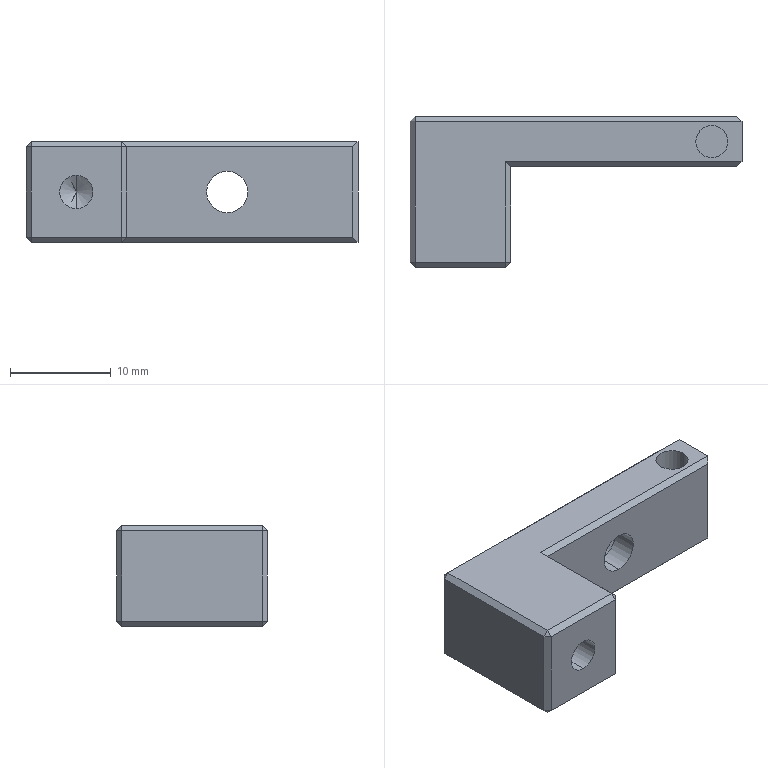Part | SolidWorks | features ICE 5, Chamfer 1, Extrusion 1, HoleWzd 1, MirrorPattern 1 | 1 solid | 44 faces | box 33 x 15 x 10 mm | volume 2355 mm3 | plane 32 | cylinder 10 | cone 2 | commonest cylinder face diameters 3.2 x4 3.3 x2 4.1 x2 7 x2
STEP:
#1=CARTESIAN_POINT('',(3.5,2.5,2.95));
#2=VERTEX_POINT('',#1);
#3=CARTESIAN_POINT('',(3.5,2.5,7.05));
#4=VERTEX_POINT('',#3);
#5=CARTESIAN_POINT('',(3.5,2.5,5.));
#6=DIRECTION('',(0.,1.,0.));
#7=DIRECTION('',(-1.,0.,0.));
#8=AXIS2_PLACEMENT_3D('',#5,#6,#7);
#9=CIRCLE('',#8,2.05);
#10=EDGE_CURVE('',#2,#4,#9,.T.);
#11=ORIENTED_EDGE('',*,*,#10,.F.);
#12=CARTESIAN_POINT('',(3.5,5.,2.95));
#13=VERTEX_POINT('',#12);
#14=CARTESIAN_POINT('',(3.5,-5.,2.95));
#15=DIRECTION('',(0.,1.,0.));
#16=VECTOR('',#15,1000.);
#17=LINE('',#14,#16);
#18=EDGE_CURVE('',#2,#13,#17,.T.);
#19=ORIENTED_EDGE('',*,*,#18,.T.);
#20=CARTESIAN_POINT('',(3.5,5.,7.05));
#21=VERTEX_POINT('',#20);
#22=CARTESIAN_POINT('',(3.5,5.,5.));
#23=DIRECTION('',(0.,1.,0.));
#24=DIRECTION('',(0.,0.,1.));
#25=AXIS2_PLACEMENT_3D('',#22,#23,#24);
#26=CIRCLE('',#25,2.05);
#27=EDGE_CURVE('',#13,#21,#26,.T.);
#28=ORIENTED_EDGE('',*,*,#27,.T.);
#29=CARTESIAN_POINT('',(3.5,-5.,7.05));
#30=DIRECTION('',(0.,1.,0.));
#31=VECTOR('',#30,1000.);
#32=LINE('',#29,#31);
#33=EDGE_CURVE('',#4,#21,#32,.T.);
#34=ORIENTED_EDGE('',*,*,#33,.F.);
#35=EDGE_LOOP('',(#11,#19,#28,#34));
#36=FACE_OUTER_BOUND('',#35,.T.);
#37=CARTESIAN_POINT('',(3.5,-5.,5.));
#38=DIRECTION('',(0.,1.,0.));
#39=DIRECTION('',(0.,0.,1.));
#40=AXIS2_PLACEMENT_3D('',#37,#38,#39);
#41=CYLINDRICAL_SURFACE('',#40,2.05);
#42=ADVANCED_FACE('',(#36),#41,.F.);
#43=CARTESIAN_POINT('',(15.1,5.,7.));
#44=VERTEX_POINT('',#43);
#45=CARTESIAN_POINT('',(11.9,5.,7.));
#46=VERTEX_POINT('',#45);
#47=CARTESIAN_POINT('',(13.5,5.,7.));
#48=DIRECTION('',(0.,0.,-1.));
#49=DIRECTION('',(-1.,0.,0.));
#50=AXIS2_PLACEMENT_3D('',#47,#48,#49);
#51=CIRCLE('',#50,1.6);
#52=EDGE_CURVE('',#44,#46,#51,.T.);
#53=ORIENTED_EDGE('',*,*,#52,.T.);
#54=CARTESIAN_POINT('',(11.9,5.,10.));
#55=VERTEX_POINT('',#54);
#56=CARTESIAN_POINT('',(11.9,5.,7.));
#57=DIRECTION('',(0.,0.,1.));
#58=VECTOR('',#57,1000.);
#59=LINE('',#56,#58);
#60=EDGE_CURVE('',#46,#55,#59,.T.);
#61=ORIENTED_EDGE('',*,*,#60,.T.);
#62=CARTESIAN_POINT('',(15.1,5.,10.));
#63=VERTEX_POINT('',#62);
#64=CARTESIAN_POINT('',(13.5,5.,10.));
#65=DIRECTION('',(0.,0.,-1.));
#66=DIRECTION('',(-1.,0.,0.));
#67=AXIS2_PLACEMENT_3D('',#64,#65,#66);
#68=CIRCLE('',#67,1.6);
#69=EDGE_CURVE('',#63,#55,#68,.T.);
#70=ORIENTED_EDGE('',*,*,#69,.F.);
#71=CARTESIAN_POINT('',(15.1,5.,7.));
#72=DIRECTION('',(0.,0.,1.));
#73=VECTOR('',#72,1000.);
#74=LINE('',#71,#73);
#75=EDGE_CURVE('',#44,#63,#74,.T.);
#76=ORIENTED_EDGE('',*,*,#75,.F.);
#77=EDGE_LOOP('',(#53,#61,#70,#76));
#78=FACE_OUTER_BOUND('',#77,.T.);
#79=CARTESIAN_POINT('',(13.5,5.,7.));
#80=DIRECTION('',(0.,0.,1.));
#81=DIRECTION('',(1.,0.,0.));
#82=AXIS2_PLACEMENT_3D('',#79,#80,#81);
#83=CYLINDRICAL_SURFACE('',#82,1.6);
#84=ADVANCED_FACE('',(#78),#83,.F.);
#85=CARTESIAN_POINT('',(15.1,5.,3.));
#86=VERTEX_POINT('',#85);
#87=CARTESIAN_POINT('',(11.9,5.,3.));
#88=VERTEX_POINT('',#87);
#89=CARTESIAN_POINT('',(13.5,5.,3.));
#90=DIRECTION('',(0.,0.,-1.));
#91=DIRECTION('',(-1.,0.,0.));
#92=AXIS2_PLACEMENT_3D('',#89,#90,#91);
#93=CIRCLE('',#92,1.6);
#94=EDGE_CURVE('',#86,#88,#93,.T.);
#95=ORIENTED_EDGE('',*,*,#94,.F.);
#96=CARTESIAN_POINT('',(15.1,5.,0.));
#97=VERTEX_POINT('',#96);
#98=CARTESIAN_POINT('',(15.1,5.,3.));
#99=DIRECTION('',(0.,0.,-1.));
#100=VECTOR('',#99,1000.);
#101=LINE('',#98,#100);
#102=EDGE_CURVE('',#86,#97,#101,.T.);
#103=ORIENTED_EDGE('',*,*,#102,.T.);
#104=CARTESIAN_POINT('',(11.9,5.,0.));
#105=VERTEX_POINT('',#104);
#106=CARTESIAN_POINT('',(13.5,5.,0.));
#107=DIRECTION('',(0.,0.,-1.));
#108=DIRECTION('',(-1.,0.,0.));
#109=AXIS2_PLACEMENT_3D('',#106,#107,#108);
#110=CIRCLE('',#109,1.6);
#111=EDGE_CURVE('',#97,#105,#110,.T.);
#112=ORIENTED_EDGE('',*,*,#111,.T.);
#113=CARTESIAN_POINT('',(11.9,5.,3.));
#114=DIRECTION('',(0.,0.,-1.));
#115=VECTOR('',#114,1000.);
#116=LINE('',#113,#115);
#117=EDGE_CURVE('',#88,#105,#116,.T.);
#118=ORIENTED_EDGE('',*,*,#117,.F.);
#119=EDGE_LOOP('',(#95,#103,#112,#118));
#120=FACE_OUTER_BOUND('',#119,.T.);
#121=CARTESIAN_POINT('',(13.5,5.,3.));
#122=DIRECTION('',(0.,0.,-1.));
#123=DIRECTION('',(-1.,0.,0.));
#124=AXIS2_PLACEMENT_3D('',#121,#122,#123);
#125=CYLINDRICAL_SURFACE('',#124,1.6);
#126=ADVANCED_FACE('',(#120),#125,.F.);
#127=CARTESIAN_POINT('',(3.5,5.,1.5));
#128=VERTEX_POINT('',#127);
#129=CARTESIAN_POINT('',(3.5,5.,8.5));
#130=VERTEX_POINT('',#129);
#131=CARTESIAN_POINT('',(3.5,5.,5.));
#132=DIRECTION('',(0.,1.,0.));
#133=DIRECTION('',(0.,0.,1.));
#134=AXIS2_PLACEMENT_3D('',#131,#132,#133);
#135=CIRCLE('',#134,3.5);
#136=EDGE_CURVE('',#128,#130,#135,.T.);
#137=ORIENTED_EDGE('',*,*,#136,.F.);
#138=CARTESIAN_POINT('',(3.5,7.5,1.5));
#139=VERTEX_POINT('',#138);
#140=CARTESIAN_POINT('',(3.5,5.,1.5));
#141=DIRECTION('',(0.,1.,0.));
#142=VECTOR('',#141,1000.);
#143=LINE('',#140,#142);
#144=EDGE_CURVE('',#128,#139,#143,.T.);
#145=ORIENTED_EDGE('',*,*,#144,.T.);
#146=CARTESIAN_POINT('',(3.5,7.5,8.5));
#147=VERTEX_POINT('',#146);
#148=CARTESIAN_POINT('',(3.5,7.5,5.));
#149=DIRECTION('',(0.,1.,0.));
#150=DIRECTION('',(0.,0.,1.));
#151=AXIS2_PLACEMENT_3D('',#148,#149,#150);
#152=CIRCLE('',#151,3.5);
#153=EDGE_CURVE('',#139,#147,#152,.T.);
#154=ORIENTED_EDGE('',*,*,#153,.T.);
#155=CARTESIAN_POINT('',(3.5,5.,8.5));
#156=DIRECTION('',(0.,1.,0.));
#157=VECTOR('',#156,1000.);
#158=LINE('',#155,#157);
#159=EDGE_CURVE('',#130,#147,#158,.T.);
#160=ORIENTED_EDGE('',*,*,#159,.F.);
#161=EDGE_LOOP('',(#137,#145,#154,#160));
#162=FACE_OUTER_BOUND('',#161,.T.);
#163=CARTESIAN_POINT('',(3.5,5.,5.));
#164=DIRECTION('',(0.,1.,0.));
#165=DIRECTION('',(0.,0.,1.));
#166=AXIS2_PLACEMENT_3D('',#163,#164,#165);
#167=CYLINDRICAL_SURFACE('',#166,3.5);
#168=ADVANCED_FACE('',(#162),#167,.F.);
#169=CARTESIAN_POINT('',(-11.5,2.6,6.65));
#170=VERTEX_POINT('',#169);
#171=CARTESIAN_POINT('',(-11.5,2.6,3.35));
#172=VERTEX_POINT('',#171);
#173=CARTESIAN_POINT('',(-11.5,2.6,5.));
#174=DIRECTION('',(0.,-1.,0.));
#175=DIRECTION('',(0.,0.,-1.));
#176=AXIS2_PLACEMENT_3D('',#173,#174,#175);
#177=CIRCLE('',#176,1.65);
#178=EDGE_CURVE('',#170,#172,#177,.T.);
#179=ORIENTED_EDGE('',*,*,#178,.F.);
#180=CARTESIAN_POINT('',(-11.5,-7.5,6.65));
#181=VERTEX_POINT('',#180);
#182=CARTESIAN_POINT('',(-11.5,-7.5,6.65));
#183=DIRECTION('',(0.,-1.,0.));
#184=VECTOR('',#183,1000.);
#185=LINE('',#182,#184);
#186=EDGE_CURVE('',#170,#181,#185,.T.);
#187=ORIENTED_EDGE('',*,*,#186,.T.);
#188=CARTESIAN_POINT('',(-11.5,-7.5,3.35));
#189=VERTEX_POINT('',#188);
#190=CARTESIAN_POINT('',(-11.5,-7.5,5.));
#191=DIRECTION('',(0.,-1.,0.));
#192=DIRECTION('',(0.,0.,-1.));
#193=AXIS2_PLACEMENT_3D('',#190,#191,#192);
#194=CIRCLE('',#193,1.65);
#195=EDGE_CURVE('',#181,#189,#194,.T.);
#196=ORIENTED_EDGE('',*,*,#195,.T.);
#197=CARTESIAN_POINT('',(-11.5,-7.5,3.35));
#198=DIRECTION('',(0.,-1.,0.));
#199=VECTOR('',#198,1000.);
#200=LINE('',#197,#199);
#201=EDGE_CURVE('',#172,#189,#200,.T.);
#202=ORIENTED_EDGE('',*,*,#201,.F.);
#203=EDGE_LOOP('',(#179,#187,#196,#202));
#204=FACE_OUTER_BOUND('',#203,.T.);
#205=CARTESIAN_POINT('',(-11.5,-7.5,5.));
#206=DIRECTION('',(0.,-1.,0.));
#207=DIRECTION('',(0.,0.,-1.));
#208=AXIS2_PLACEMENT_3D('',#205,#206,#207);
#209=CYLINDRICAL_SURFACE('',#208,1.65);
#210=ADVANCED_FACE('',(#204),#209,.F.);
#211=CARTESIAN_POINT('',(-11.5,3.591,5.));
#212=VERTEX_POINT('',#211);
#213=CARTESIAN_POINT('',(-11.5,2.6,3.35));
#214=DIRECTION('',(0.,-0.515,-0.8572));
#215=VECTOR('',#214,1000.);
#216=LINE('',#213,#215);
#217=EDGE_CURVE('',#212,#172,#216,.T.);
#218=ORIENTED_EDGE('',*,*,#217,.F.);
#219=CARTESIAN_POINT('',(-11.5,2.6,6.65));
#220=DIRECTION('',(0.,-0.515,0.8572));
#221=VECTOR('',#220,1000.);
#222=LINE('',#219,#221);
#223=EDGE_CURVE('',#212,#170,#222,.T.);
#224=ORIENTED_EDGE('',*,*,#223,.T.);
#225=ORIENTED_EDGE('',*,*,#178,.T.);
#226=EDGE_LOOP('',(#218,#224,#225));
#227=FACE_OUTER_BOUND('',#226,.T.);
#228=CARTESIAN_POINT('',(-11.5,2.6,5.));
#229=DIRECTION('',(0.,-1.,0.));
#230=DIRECTION('',(0.,0.,-1.));
#231=AXIS2_PLACEMENT_3D('',#228,#229,#230);
#232=CONICAL_SURFACE('',#231,1.65,1.03);
#233=ADVANCED_FACE('',(#227),#232,.F.);
#234=CARTESIAN_POINT('',(16.5,3.,10.));
#235=VERTEX_POINT('',#234);
#236=CARTESIAN_POINT('',(16.5,7.,10.));
#237=VERTEX_POINT('',#236);
#238=CARTESIAN_POINT('',(16.5,-7.5,10.));
#239=DIRECTION('',(0.,1.,0.));
#240=VECTOR('',#239,1000.);
#241=LINE('',#238,#240);
#242=EDGE_CURVE('',#235,#237,#241,.T.);
#243=ORIENTED_EDGE('',*,*,#242,.T.);
#244=CARTESIAN_POINT('',(-16.,7.,10.));
#245=VERTEX_POINT('',#244);
#246=CARTESIAN_POINT('',(0.,7.,10.));
#247=DIRECTION('',(-1.,0.,0.));
#248=VECTOR('',#247,1000.);
#249=LINE('',#246,#248);
#250=EDGE_CURVE('',#237,#245,#249,.T.);
#251=ORIENTED_EDGE('',*,*,#250,.T.);
#252=CARTESIAN_POINT('',(-16.,-7.,10.));
#253=VERTEX_POINT('',#252);
#254=CARTESIAN_POINT('',(-16.,0.,10.));
#255=DIRECTION('',(0.,-1.,0.));
#256=VECTOR('',#255,1000.);
#257=LINE('',#254,#256);
#258=EDGE_CURVE('',#245,#253,#257,.T.);
#259=ORIENTED_EDGE('',*,*,#258,.T.);
#260=CARTESIAN_POINT('',(-7.,-7.,10.));
#261=VERTEX_POINT('',#260);
#262=CARTESIAN_POINT('',(0.,-7.,10.));
#263=DIRECTION('',(1.,0.,0.));
#264=VECTOR('',#263,1000.);
#265=LINE('',#262,#264);
#266=EDGE_CURVE('',#253,#261,#265,.T.);
#267=ORIENTED_EDGE('',*,*,#266,.T.);
#268=CARTESIAN_POINT('',(-7.,3.,10.));
#269=VERTEX_POINT('',#268);
#270=CARTESIAN_POINT('',(-7.,0.,10.));
#271=DIRECTION('',(0.,1.,0.));
#272=VECTOR('',#271,1000.);
#273=LINE('',#270,#272);
#274=EDGE_CURVE('',#261,#269,#273,.T.);
#275=ORIENTED_EDGE('',*,*,#274,.T.);
#276=CARTESIAN_POINT('',(0.,3.,10.));
#277=DIRECTION('',(1.,0.,0.));
#278=VECTOR('',#277,1000.);
#279=LINE('',#276,#278);
#280=EDGE_CURVE('',#269,#235,#279,.T.);
#281=ORIENTED_EDGE('',*,*,#280,.T.);
#282=EDGE_LOOP('',(#243,#251,#259,#267,#275,#281));
#283=FACE_OUTER_BOUND('',#282,.T.);
#284=ORIENTED_EDGE('',*,*,#69,.T.);
#285=CARTESIAN_POINT('',(13.5,5.,10.));
#286=DIRECTION('',(0.,0.,-1.));
#287=DIRECTION('',(-1.,0.,0.));
#288=AXIS2_PLACEMENT_3D('',#285,#286,#287);
#289=CIRCLE('',#288,1.6);
#290=EDGE_CURVE('',#55,#63,#289,.T.);
#291=ORIENTED_EDGE('',*,*,#290,.T.);
#292=EDGE_LOOP('',(#284,#291));
#293=FACE_BOUND('',#292,.T.);
#294=CARTESIAN_POINT('',(0.,0.,10.));
#295=DIRECTION('',(0.,0.,-1.));
#296=DIRECTION('',(-1.,0.,0.));
#297=AXIS2_PLACEMENT_3D('',#294,#295,#296);
#298=PLANE('',#297);
#299=ADVANCED_FACE('',(#283,#293),#298,.F.);
#300=CARTESIAN_POINT('',(16.5,3.,0.));
#301=VERTEX_POINT('',#300);
#302=CARTESIAN_POINT('',(16.5,7.,0.));
#303=VERTEX_POINT('',#302);
#304=CARTESIAN_POINT('',(16.5,-7.5,0.));
#305=DIRECTION('',(0.,1.,0.));
#306=VECTOR('',#305,1000.);
#307=LINE('',#304,#306);
#308=EDGE_CURVE('',#301,#303,#307,.T.);
#309=ORIENTED_EDGE('',*,*,#308,.T.);
#310=CARTESIAN_POINT('',(16.5,7.,10.));
#311=DIRECTION('',(0.,0.,1.));
#312=VECTOR('',#311,1000.);
#313=LINE('',#310,#312);
#314=EDGE_CURVE('',#303,#237,#313,.T.);
#315=ORIENTED_EDGE('',*,*,#314,.T.);
#316=ORIENTED_EDGE('',*,*,#242,.F.);
#317=CARTESIAN_POINT('',(16.5,3.,10.));
#318=DIRECTION('',(0.,0.,-1.));
#319=VECTOR('',#318,1000.);
#320=LINE('',#317,#319);
#321=EDGE_CURVE('',#235,#301,#320,.T.);
#322=ORIENTED_EDGE('',*,*,#321,.T.);
#323=EDGE_LOOP('',(#309,#315,#316,#322));
#324=FACE_OUTER_BOUND('',#323,.T.);
#325=CARTESIAN_POINT('',(16.5,-7.5,10.));
#326=DIRECTION('',(-1.,0.,0.));
#327=DIRECTION('',(0.,0.,1.));
#328=AXIS2_PLACEMENT_3D('',#325,#326,#327);
#329=PLANE('',#328);
#330=ADVANCED_FACE('',(#324),#329,.F.);
#331=CARTESIAN_POINT('',(3.5,7.5,5.));
#332=DIRECTION('',(0.,1.,0.));
#333=DIRECTION('',(0.,0.,1.));
#334=AXIS2_PLACEMENT_3D('',#331,#332,#333);
#335=CIRCLE('',#334,3.5);
#336=EDGE_CURVE('',#147,#139,#335,.T.);
#337=ORIENTED_EDGE('',*,*,#336,.F.);
#338=ORIENTED_EDGE('',*,*,#153,.F.);
#339=EDGE_LOOP('',(#337,#338));
#340=FACE_BOUND('',#339,.T.);
#341=CARTESIAN_POINT('',(-16.,7.5,0.5));
#342=VERTEX_POINT('',#341);
#343=CARTESIAN_POINT('',(-16.,7.5,9.5));
#344=VERTEX_POINT('',#343);
#345=CARTESIAN_POINT('',(-16.,7.5,10.));
#346=DIRECTION('',(0.,0.,1.));
#347=VECTOR('',#346,1000.);
#348=LINE('',#345,#347);
#349=EDGE_CURVE('',#342,#344,#348,.T.);
#350=ORIENTED_EDGE('',*,*,#349,.T.);
#351=CARTESIAN_POINT('',(16.,7.5,9.5));
#352=VERTEX_POINT('',#351);
#353=CARTESIAN_POINT('',(-16.5,7.5,9.5));
#354=DIRECTION('',(1.,0.,0.));
#355=VECTOR('',#354,1000.);
#356=LINE('',#353,#355);
#357=EDGE_CURVE('',#344,#352,#356,.T.);
#358=ORIENTED_EDGE('',*,*,#357,.T.);
#359=CARTESIAN_POINT('',(16.,7.5,0.5));
#360=VERTEX_POINT('',#359);
#361=CARTESIAN_POINT('',(16.,7.5,10.));
#362=DIRECTION('',(0.,0.,-1.));
#363=VECTOR('',#362,1000.);
#364=LINE('',#361,#363);
#365=EDGE_CURVE('',#352,#360,#364,.T.);
#366=ORIENTED_EDGE('',*,*,#365,.T.);
#367=CARTESIAN_POINT('',(-16.5,7.5,0.5));
#368=DIRECTION('',(-1.,0.,0.));
#369=VECTOR('',#368,1000.);
#370=LINE('',#367,#369);
#371=EDGE_CURVE('',#360,#342,#370,.T.);
#372=ORIENTED_EDGE('',*,*,#371,.T.);
#373=EDGE_LOOP('',(#350,#358,#366,#372));
#374=FACE_OUTER_BOUND('',#373,.T.);
#375=CARTESIAN_POINT('',(-16.5,7.5,10.));
#376=DIRECTION('',(0.,-1.,0.));
#377=DIRECTION('',(0.,0.,-1.));
#378=AXIS2_PLACEMENT_3D('',#375,#376,#377);
#379=PLANE('',#378);
#380=ADVANCED_FACE('',(#340,#374),#379,.F.);
#381=CARTESIAN_POINT('',(-16.5,-7.,9.5));
#382=VERTEX_POINT('',#381);
#383=CARTESIAN_POINT('',(-16.5,7.,9.5));
#384=VERTEX_POINT('',#383);
#385=CARTESIAN_POINT('',(-16.5,-7.5,9.5));
#386=DIRECTION('',(0.,1.,0.));
#387=VECTOR('',#386,1000.);
#388=LINE('',#385,#387);
#389=EDGE_CURVE('',#382,#384,#388,.T.);
#390=ORIENTED_EDGE('',*,*,#389,.T.);
#391=CARTESIAN_POINT('',(-16.5,7.,0.5));
#392=VERTEX_POINT('',#391);
#393=CARTESIAN_POINT('',(-16.5,7.,10.));
#394=DIRECTION('',(0.,0.,-1.));
#395=VECTOR('',#394,1000.);
#396=LINE('',#393,#395);
#397=EDGE_CURVE('',#384,#392,#396,.T.);
#398=ORIENTED_EDGE('',*,*,#397,.T.);
#399=CARTESIAN_POINT('',(-16.5,-7.,0.5));
#400=VERTEX_POINT('',#399);
#401=CARTESIAN_POINT('',(-16.5,-7.5,0.5));
#402=DIRECTION('',(0.,-1.,0.));
#403=VECTOR('',#402,1000.);
#404=LINE('',#401,#403);
#405=EDGE_CURVE('',#392,#400,#404,.T.);
#406=ORIENTED_EDGE('',*,*,#405,.T.);
#407=CARTESIAN_POINT('',(-16.5,-7.,10.));
#408=DIRECTION('',(0.,0.,1.));
#409=VECTOR('',#408,1000.);
#410=LINE('',#407,#409);
#411=EDGE_CURVE('',#400,#382,#410,.T.);
#412=ORIENTED_EDGE('',*,*,#411,.T.);
#413=EDGE_LOOP('',(#390,#398,#406,#412));
#414=FACE_OUTER_BOUND('',#413,.T.);
#415=CARTESIAN_POINT('',(-16.5,-7.5,10.));
#416=DIRECTION('',(1.,0.,0.));
#417=DIRECTION('',(0.,0.,-1.));
#418=AXIS2_PLACEMENT_3D('',#415,#416,#417);
#419=PLANE('',#418);
#420=ADVANCED_FACE('',(#414),#419,.F.);
#421=CARTESIAN_POINT('',(-16.,-7.5,9.5));
#422=VERTEX_POINT('',#421);
#423=CARTESIAN_POINT('',(-16.,-7.5,0.5));
#424=VERTEX_POINT('',#423);
#425=CARTESIAN_POINT('',(-16.,-7.5,10.));
#426=DIRECTION('',(0.,0.,-1.));
#427=VECTOR('',#426,1000.);
#428=LINE('',#425,#427);
#429=EDGE_CURVE('',#422,#424,#428,.T.);
#430=ORIENTED_EDGE('',*,*,#429,.T.);
#431=CARTESIAN_POINT('',(-7.,-7.5,0.5));
#432=VERTEX_POINT('',#431);
#433=CARTESIAN_POINT('',(-6.5,-7.5,0.5));
#434=DIRECTION('',(1.,0.,0.));
#435=VECTOR('',#434,1000.);
#436=LINE('',#433,#435);
#437=EDGE_CURVE('',#424,#432,#436,.T.);
#438=ORIENTED_EDGE('',*,*,#437,.T.);
#439=CARTESIAN_POINT('',(-7.,-7.5,9.5));
#440=VERTEX_POINT('',#439);
#441=CARTESIAN_POINT('',(-7.,-7.5,10.));
#442=DIRECTION('',(0.,0.,1.));
#443=VECTOR('',#442,1000.);
#444=LINE('',#441,#443);
#445=EDGE_CURVE('',#432,#440,#444,.T.);
#446=ORIENTED_EDGE('',*,*,#445,.T.);
#447=CARTESIAN_POINT('',(-16.5,-7.5,9.5));
#448=DIRECTION('',(-1.,0.,0.));
#449=VECTOR('',#448,1000.);
#450=LINE('',#447,#449);
#451=EDGE_CURVE('',#440,#422,#450,.T.);
#452=ORIENTED_EDGE('',*,*,#451,.T.);
#453=EDGE_LOOP('',(#430,#438,#446,#452));
#454=FACE_OUTER_BOUND('',#453,.T.);
#455=CARTESIAN_POINT('',(-11.5,-7.5,5.));
#456=DIRECTION('',(0.,-1.,0.));
#457=DIRECTION('',(0.,0.,-1.));
#458=AXIS2_PLACEMENT_3D('',#455,#456,#457);
#459=CIRCLE('',#458,1.65);
#460=EDGE_CURVE('',#189,#181,#459,.T.);
#461=ORIENTED_EDGE('',*,*,#460,.F.);
#462=ORIENTED_EDGE('',*,*,#195,.F.);
#463=EDGE_LOOP('',(#461,#462));
#464=FACE_BOUND('',#463,.T.);
#465=CARTESIAN_POINT('',(-16.5,-7.5,10.));
#466=DIRECTION('',(0.,1.,0.));
#467=DIRECTION('',(0.,0.,1.));
#468=AXIS2_PLACEMENT_3D('',#465,#466,#467);
#469=PLANE('',#468);
#470=ADVANCED_FACE('',(#454,#464),#469,.F.);
#471=CARTESIAN_POINT('',(13.5,5.,0.));
#472=DIRECTION('',(0.,0.,-1.));
#473=DIRECTION('',(-1.,0.,0.));
#474=AXIS2_PLACEMENT_3D('',#471,#472,#473);
#475=CIRCLE('',#474,1.6);
#476=EDGE_CURVE('',#105,#97,#475,.T.);
#477=ORIENTED_EDGE('',*,*,#476,.F.);
#478=ORIENTED_EDGE('',*,*,#111,.F.);
#479=EDGE_LOOP('',(#477,#478));
#480=FACE_BOUND('',#479,.T.);
#481=CARTESIAN_POINT('',(-16.,-7.,0.));
#482=VERTEX_POINT('',#481);
#483=CARTESIAN_POINT('',(-16.,7.,0.));
#484=VERTEX_POINT('',#483);
#485=CARTESIAN_POINT('',(-16.,7.5,0.));
#486=DIRECTION('',(0.,1.,0.));
#487=VECTOR('',#486,1000.);
#488=LINE('',#485,#487);
#489=EDGE_CURVE('',#482,#484,#488,.T.);
#490=ORIENTED_EDGE('',*,*,#489,.T.);
#491=CARTESIAN_POINT('',(16.5,7.,0.));
#492=DIRECTION('',(1.,0.,0.));
#493=VECTOR('',#492,1000.);
#494=LINE('',#491,#493);
#495=EDGE_CURVE('',#484,#303,#494,.T.);
#496=ORIENTED_EDGE('',*,*,#495,.T.);
#497=ORIENTED_EDGE('',*,*,#308,.F.);
#498=CARTESIAN_POINT('',(-7.,3.,0.));
#499=VERTEX_POINT('',#498);
#500=CARTESIAN_POINT('',(-6.5,3.,0.));
#501=DIRECTION('',(-1.,0.,0.));
#502=VECTOR('',#501,1000.);
#503=LINE('',#500,#502);
#504=EDGE_CURVE('',#301,#499,#503,.T.);
#505=ORIENTED_EDGE('',*,*,#504,.T.);
#506=CARTESIAN_POINT('',(-7.,-7.,0.));
#507=VERTEX_POINT('',#506);
#508=CARTESIAN_POINT('',(-7.,-7.5,0.));
#509=DIRECTION('',(0.,-1.,0.));
#510=VECTOR('',#509,1000.);
#511=LINE('',#508,#510);
#512=EDGE_CURVE('',#499,#507,#511,.T.);
#513=ORIENTED_EDGE('',*,*,#512,.T.);
#514=CARTESIAN_POINT('',(-16.5,-7.,0.));
#515=DIRECTION('',(-1.,0.,0.));
#516=VECTOR('',#515,1000.);
#517=LINE('',#514,#516);
#518=EDGE_CURVE('',#507,#482,#517,.T.);
#519=ORIENTED_EDGE('',*,*,#518,.T.);
#520=EDGE_LOOP('',(#490,#496,#497,#505,#513,#519));
#521=FACE_OUTER_BOUND('',#520,.T.);
#522=CARTESIAN_POINT('',(0.,0.,0.));
#523=DIRECTION('',(0.,0.,-1.));
#524=DIRECTION('',(-1.,0.,0.));
#525=AXIS2_PLACEMENT_3D('',#522,#523,#524);
#526=PLANE('',#525);
#527=ADVANCED_FACE('',(#480,#521),#526,.T.);
#528=CARTESIAN_POINT('',(-6.5,2.5,0.5));
#529=VERTEX_POINT('',#528);
#530=CARTESIAN_POINT('',(-6.5,2.5,9.5));
#531=VERTEX_POINT('',#530);
#532=CARTESIAN_POINT('',(-6.5,2.5,-10.));
#533=DIRECTION('',(0.,0.,1.));
#534=VECTOR('',#533,1000.);
#535=LINE('',#532,#534);
#536=EDGE_CURVE('',#529,#531,#535,.T.);
#537=ORIENTED_EDGE('',*,*,#536,.T.);
#538=CARTESIAN_POINT('',(-6.5,-7.,9.5));
#539=VERTEX_POINT('',#538);
#540=CARTESIAN_POINT('',(-6.5,-7.5,9.5));
#541=DIRECTION('',(0.,-1.,0.));
#542=VECTOR('',#541,1000.);
#543=LINE('',#540,#542);
#544=EDGE_CURVE('',#531,#539,#543,.T.);
#545=ORIENTED_EDGE('',*,*,#544,.T.);
#546=CARTESIAN_POINT('',(-6.5,-7.,0.5));
#547=VERTEX_POINT('',#546);
#548=CARTESIAN_POINT('',(-6.5,-7.,-10.));
#549=DIRECTION('',(0.,0.,-1.));
#550=VECTOR('',#549,1000.);
#551=LINE('',#548,#550);
#552=EDGE_CURVE('',#539,#547,#551,.T.);
#553=ORIENTED_EDGE('',*,*,#552,.T.);
#554=CARTESIAN_POINT('',(-6.5,2.5,0.5));
#555=DIRECTION('',(0.,1.,0.));
#556=VECTOR('',#555,1000.);
#557=LINE('',#554,#556);
#558=EDGE_CURVE('',#547,#529,#557,.T.);
#559=ORIENTED_EDGE('',*,*,#558,.T.);
#560=EDGE_LOOP('',(#537,#545,#553,#559));
#561=FACE_OUTER_BOUND('',#560,.T.);
#562=CARTESIAN_POINT('',(-6.5,-7.5,-10.));
#563=DIRECTION('',(-1.,0.,0.));
#564=DIRECTION('',(0.,0.,1.));
#565=AXIS2_PLACEMENT_3D('',#562,#563,#564);
#566=PLANE('',#565);
#567=ADVANCED_FACE('',(#561),#566,.F.);
#568=CARTESIAN_POINT('',(3.5,2.5,5.));
#569=DIRECTION('',(0.,1.,0.));
#570=DIRECTION('',(-1.,0.,0.));
#571=AXIS2_PLACEMENT_3D('',#568,#569,#570);
#572=CIRCLE('',#571,2.05);
#573=EDGE_CURVE('',#4,#2,#572,.T.);
#574=ORIENTED_EDGE('',*,*,#573,.T.);
#575=ORIENTED_EDGE('',*,*,#10,.T.);
#576=EDGE_LOOP('',(#574,#575));
#577=FACE_BOUND('',#576,.T.);
#578=ORIENTED_EDGE('',*,*,#536,.F.);
#579=CARTESIAN_POINT('',(16.,2.5,0.5));
#580=VERTEX_POINT('',#579);
#581=CARTESIAN_POINT('',(16.5,2.5,0.5));
#582=DIRECTION('',(1.,0.,0.));
#583=VECTOR('',#582,1000.);
#584=LINE('',#581,#583);
#585=EDGE_CURVE('',#529,#580,#584,.T.);
#586=ORIENTED_EDGE('',*,*,#585,.T.);
#587=CARTESIAN_POINT('',(16.,2.5,9.5));
#588=VERTEX_POINT('',#587);
#589=CARTESIAN_POINT('',(16.,2.5,-10.));
#590=DIRECTION('',(0.,0.,1.));
#591=VECTOR('',#590,1000.);
#592=LINE('',#589,#591);
#593=EDGE_CURVE('',#580,#588,#592,.T.);
#594=ORIENTED_EDGE('',*,*,#593,.T.);
#595=CARTESIAN_POINT('',(16.5,2.5,9.5));
#596=DIRECTION('',(-1.,0.,0.));
#597=VECTOR('',#596,1000.);
#598=LINE('',#595,#597);
#599=EDGE_CURVE('',#588,#531,#598,.T.);
#600=ORIENTED_EDGE('',*,*,#599,.T.);
#601=EDGE_LOOP('',(#578,#586,#594,#600));
#602=FACE_OUTER_BOUND('',#601,.T.);
#603=CARTESIAN_POINT('',(16.5,2.5,-10.));
#604=DIRECTION('',(0.,1.,0.));
#605=DIRECTION('',(-1.,0.,0.));
#606=AXIS2_PLACEMENT_3D('',#603,#604,#605);
#607=PLANE('',#606);
#608=ADVANCED_FACE('',(#577,#602),#607,.F.);
#609=ORIENTED_EDGE('',*,*,#223,.F.);
#610=ORIENTED_EDGE('',*,*,#217,.T.);
#611=CARTESIAN_POINT('',(-11.5,2.6,5.));
#612=DIRECTION('',(0.,-1.,0.));
#613=DIRECTION('',(0.,0.,-1.));
#614=AXIS2_PLACEMENT_3D('',#611,#612,#613);
#615=CIRCLE('',#614,1.65);
#616=EDGE_CURVE('',#172,#170,#615,.T.);
#617=ORIENTED_EDGE('',*,*,#616,.T.);
#618=EDGE_LOOP('',(#609,#610,#617));
#619=FACE_OUTER_BOUND('',#618,.T.);
#620=CARTESIAN_POINT('',(-11.5,2.6,5.));
#621=DIRECTION('',(0.,-1.,0.));
#622=DIRECTION('',(0.,0.,-1.));
#623=AXIS2_PLACEMENT_3D('',#620,#621,#622);
#624=CONICAL_SURFACE('',#623,1.65,1.03);
#625=ADVANCED_FACE('',(#619),#624,.F.);
#626=ORIENTED_EDGE('',*,*,#186,.F.);
#627=ORIENTED_EDGE('',*,*,#616,.F.);
#628=ORIENTED_EDGE('',*,*,#201,.T.);
#629=ORIENTED_EDGE('',*,*,#460,.T.);
#630=EDGE_LOOP('',(#626,#627,#628,#629));
#631=FACE_OUTER_BOUND('',#630,.T.);
#632=CARTESIAN_POINT('',(-11.5,-7.5,5.));
#633=DIRECTION('',(0.,-1.,0.));
#634=DIRECTION('',(0.,0.,-1.));
#635=AXIS2_PLACEMENT_3D('',#632,#633,#634);
#636=CYLINDRICAL_SURFACE('',#635,1.65);
#637=ADVANCED_FACE('',(#631),#636,.F.);
#638=CARTESIAN_POINT('',(1.167,-5.167,8.167));
#639=DIRECTION('',(0.5774,-0.5774,0.5774));
#640=VECTOR('',#639,1000.);
#641=LINE('',#638,#640);
#642=EDGE_CURVE('',#499,#529,#641,.T.);
#643=ORIENTED_EDGE('',*,*,#642,.F.);
#644=ORIENTED_EDGE('',*,*,#504,.F.);
#645=CARTESIAN_POINT('',(16.167,2.667,0.3333));
#646=DIRECTION('',(0.5774,0.5774,-0.5774));
#647=VECTOR('',#646,1000.);
#648=LINE('',#645,#647);
#649=EDGE_CURVE('',#580,#301,#648,.T.);
#650=ORIENTED_EDGE('',*,*,#649,.F.);
#651=ORIENTED_EDGE('',*,*,#585,.F.);
#652=EDGE_LOOP('',(#643,#644,#650,#651));
#653=FACE_OUTER_BOUND('',#652,.T.);
#654=CARTESIAN_POINT('',(16.5,2.5,0.5));
#655=DIRECTION('',(0.,-0.7071,-0.7071));
#656=DIRECTION('',(-1.,0.,0.));
#657=AXIS2_PLACEMENT_3D('',#654,#655,#656);
#658=PLANE('',#657);
#659=ADVANCED_FACE('',(#653),#658,.T.);
#660=ORIENTED_EDGE('',*,*,#649,.T.);
#661=ORIENTED_EDGE('',*,*,#321,.F.);
#662=CARTESIAN_POINT('',(16.167,2.667,9.667));
#663=DIRECTION('',(0.5774,0.5774,0.5774));
#664=VECTOR('',#663,1000.);
#665=LINE('',#662,#664);
#666=EDGE_CURVE('',#588,#235,#665,.T.);
#667=ORIENTED_EDGE('',*,*,#666,.F.);
#668=ORIENTED_EDGE('',*,*,#593,.F.);
#669=EDGE_LOOP('',(#660,#661,#667,#668));
#670=FACE_OUTER_BOUND('',#669,.T.);
#671=CARTESIAN_POINT('',(16.,2.5,-10.));
#672=DIRECTION('',(-0.7071,0.7071,0.));
#673=DIRECTION('',(0.,0.,1.));
#674=AXIS2_PLACEMENT_3D('',#671,#672,#673);
#675=PLANE('',#674);
#676=ADVANCED_FACE('',(#670),#675,.F.);
#677=ORIENTED_EDGE('',*,*,#642,.T.);
#678=ORIENTED_EDGE('',*,*,#558,.F.);
#679=CARTESIAN_POINT('',(-7.,-7.,0.));
#680=DIRECTION('',(0.7071,0.,0.7071));
#681=VECTOR('',#680,1000.);
#682=LINE('',#679,#681);
#683=EDGE_CURVE('',#507,#547,#682,.T.);
#684=ORIENTED_EDGE('',*,*,#683,.F.);
#685=ORIENTED_EDGE('',*,*,#512,.F.);
#686=EDGE_LOOP('',(#677,#678,#684,#685));
#687=FACE_OUTER_BOUND('',#686,.T.);
#688=CARTESIAN_POINT('',(-6.5,-7.5,0.5));
#689=DIRECTION('',(0.7071,0.,-0.7071));
#690=DIRECTION('',(0.,-1.,0.));
#691=AXIS2_PLACEMENT_3D('',#688,#689,#690);
#692=PLANE('',#691);
#693=ADVANCED_FACE('',(#687),#692,.T.);
#694=ORIENTED_EDGE('',*,*,#666,.T.);
#695=ORIENTED_EDGE('',*,*,#280,.F.);
#696=CARTESIAN_POINT('',(1.167,-5.167,1.833));
#697=DIRECTION('',(-0.5774,0.5774,0.5774));
#698=VECTOR('',#697,1000.);
#699=LINE('',#696,#698);
#700=EDGE_CURVE('',#531,#269,#699,.T.);
#701=ORIENTED_EDGE('',*,*,#700,.F.);
#702=ORIENTED_EDGE('',*,*,#599,.F.);
#703=EDGE_LOOP('',(#694,#695,#701,#702));
#704=FACE_OUTER_BOUND('',#703,.T.);
#705=CARTESIAN_POINT('',(16.5,2.5,9.5));
#706=DIRECTION('',(0.,0.7071,-0.7071));
#707=DIRECTION('',(-1.,0.,0.));
#708=AXIS2_PLACEMENT_3D('',#705,#706,#707);
#709=PLANE('',#708);
#710=ADVANCED_FACE('',(#704),#709,.F.);
#711=CARTESIAN_POINT('',(-7.,-7.,0.));
#712=DIRECTION('',(0.,-0.7071,0.7071));
#713=VECTOR('',#712,1000.);
#714=LINE('',#711,#713);
#715=EDGE_CURVE('',#507,#432,#714,.T.);
#716=ORIENTED_EDGE('',*,*,#715,.F.);
#717=ORIENTED_EDGE('',*,*,#683,.T.);
#718=CARTESIAN_POINT('',(-6.75,-7.25,0.5));
#719=DIRECTION('',(0.7071,0.7071,0.));
#720=VECTOR('',#719,1000.);
#721=LINE('',#718,#720);
#722=EDGE_CURVE('',#432,#547,#721,.T.);
#723=ORIENTED_EDGE('',*,*,#722,.F.);
#724=EDGE_LOOP('',(#716,#717,#723));
#725=FACE_OUTER_BOUND('',#724,.T.);
#726=CARTESIAN_POINT('',(-7.,-7.,0.));
#727=DIRECTION('',(0.5774,-0.5774,-0.5774));
#728=DIRECTION('',(-0.7071,0.,-0.7071));
#729=AXIS2_PLACEMENT_3D('',#726,#727,#728);
#730=PLANE('',#729);
#731=ADVANCED_FACE('',(#725),#730,.T.);
#732=ORIENTED_EDGE('',*,*,#700,.T.);
#733=ORIENTED_EDGE('',*,*,#274,.F.);
#734=CARTESIAN_POINT('',(-6.5,-7.,9.5));
#735=DIRECTION('',(-0.7071,0.,0.7071));
#736=VECTOR('',#735,1000.);
#737=LINE('',#734,#736);
#738=EDGE_CURVE('',#539,#261,#737,.T.);
#739=ORIENTED_EDGE('',*,*,#738,.F.);
#740=ORIENTED_EDGE('',*,*,#544,.F.);
#741=EDGE_LOOP('',(#732,#733,#739,#740));
#742=FACE_OUTER_BOUND('',#741,.T.);
#743=CARTESIAN_POINT('',(-6.5,-7.5,9.5));
#744=DIRECTION('',(-0.7071,0.,-0.7071));
#745=DIRECTION('',(0.,-1.,0.));
#746=AXIS2_PLACEMENT_3D('',#743,#744,#745);
#747=PLANE('',#746);
#748=ADVANCED_FACE('',(#742),#747,.F.);
#749=ORIENTED_EDGE('',*,*,#722,.T.);
#750=ORIENTED_EDGE('',*,*,#552,.F.);
#751=CARTESIAN_POINT('',(-6.5,-7.,9.5));
#752=DIRECTION('',(0.7071,0.7071,0.));
#753=VECTOR('',#752,1000.);
#754=LINE('',#751,#753);
#755=EDGE_CURVE('',#440,#539,#754,.T.);
#756=ORIENTED_EDGE('',*,*,#755,.F.);
#757=ORIENTED_EDGE('',*,*,#445,.F.);
#758=EDGE_LOOP('',(#749,#750,#756,#757));
#759=FACE_OUTER_BOUND('',#758,.T.);
#760=CARTESIAN_POINT('',(-7.,-7.5,10.));
#761=DIRECTION('',(-0.7071,0.7071,0.));
#762=DIRECTION('',(0.,0.,1.));
#763=AXIS2_PLACEMENT_3D('',#760,#761,#762);
#764=PLANE('',#763);
#765=ADVANCED_FACE('',(#759),#764,.F.);
#766=ORIENTED_EDGE('',*,*,#715,.T.);
#767=ORIENTED_EDGE('',*,*,#437,.F.);
#768=CARTESIAN_POINT('',(-16.,-7.,0.));
#769=DIRECTION('',(0.,-0.7071,0.7071));
#770=VECTOR('',#769,1000.);
#771=LINE('',#768,#770);
#772=EDGE_CURVE('',#482,#424,#771,.T.);
#773=ORIENTED_EDGE('',*,*,#772,.F.);
#774=ORIENTED_EDGE('',*,*,#518,.F.);
#775=EDGE_LOOP('',(#766,#767,#773,#774));
#776=FACE_OUTER_BOUND('',#775,.T.);
#777=CARTESIAN_POINT('',(-16.5,-7.5,0.5));
#778=DIRECTION('',(0.,-0.7071,-0.7071));
#779=DIRECTION('',(-1.,0.,0.));
#780=AXIS2_PLACEMENT_3D('',#777,#778,#779);
#781=PLANE('',#780);
#782=ADVANCED_FACE('',(#776),#781,.T.);
#783=ORIENTED_EDGE('',*,*,#755,.T.);
#784=ORIENTED_EDGE('',*,*,#738,.T.);
#785=CARTESIAN_POINT('',(-7.,-7.25,9.75));
#786=DIRECTION('',(0.,0.7071,0.7071));
#787=VECTOR('',#786,1000.);
#788=LINE('',#785,#787);
#789=EDGE_CURVE('',#440,#261,#788,.T.);
#790=ORIENTED_EDGE('',*,*,#789,.F.);
#791=EDGE_LOOP('',(#783,#784,#790));
#792=FACE_OUTER_BOUND('',#791,.T.);
#793=CARTESIAN_POINT('',(-6.5,-7.,9.5));
#794=DIRECTION('',(0.5774,-0.5774,0.5774));
#795=DIRECTION('',(0.,-0.7071,-0.7071));
#796=AXIS2_PLACEMENT_3D('',#793,#794,#795);
#797=PLANE('',#796);
#798=ADVANCED_FACE('',(#792),#797,.T.);
#799=CARTESIAN_POINT('',(-16.,-7.,0.));
#800=DIRECTION('',(-0.7071,0.,0.7071));
#801=VECTOR('',#800,1000.);
#802=LINE('',#799,#801);
#803=EDGE_CURVE('',#482,#400,#802,.T.);
#804=ORIENTED_EDGE('',*,*,#803,.F.);
#805=ORIENTED_EDGE('',*,*,#772,.T.);
#806=CARTESIAN_POINT('',(-16.25,-7.25,0.5));
#807=DIRECTION('',(0.7071,-0.7071,0.));
#808=VECTOR('',#807,1000.);
#809=LINE('',#806,#808);
#810=EDGE_CURVE('',#400,#424,#809,.T.);
#811=ORIENTED_EDGE('',*,*,#810,.F.);
#812=EDGE_LOOP('',(#804,#805,#811));
#813=FACE_OUTER_BOUND('',#812,.T.);
#814=CARTESIAN_POINT('',(-16.,-7.,0.));
#815=DIRECTION('',(-0.5774,-0.5774,-0.5774));
#816=DIRECTION('',(0.,0.7071,-0.7071));
#817=AXIS2_PLACEMENT_3D('',#814,#815,#816);
#818=PLANE('',#817);
#819=ADVANCED_FACE('',(#813),#818,.T.);
#820=ORIENTED_EDGE('',*,*,#789,.T.);
#821=ORIENTED_EDGE('',*,*,#266,.F.);
#822=CARTESIAN_POINT('',(-16.,-7.5,9.5));
#823=DIRECTION('',(0.,0.7071,0.7071));
#824=VECTOR('',#823,1000.);
#825=LINE('',#822,#824);
#826=EDGE_CURVE('',#422,#253,#825,.T.);
#827=ORIENTED_EDGE('',*,*,#826,.F.);
#828=ORIENTED_EDGE('',*,*,#451,.F.);
#829=EDGE_LOOP('',(#820,#821,#827,#828));
#830=FACE_OUTER_BOUND('',#829,.T.);
#831=CARTESIAN_POINT('',(0.,-7.,10.));
#832=DIRECTION('',(0.,0.7071,-0.7071));
#833=DIRECTION('',(1.,0.,0.));
#834=AXIS2_PLACEMENT_3D('',#831,#832,#833);
#835=PLANE('',#834);
#836=ADVANCED_FACE('',(#830),#835,.F.);
#837=ORIENTED_EDGE('',*,*,#810,.T.);
#838=ORIENTED_EDGE('',*,*,#429,.F.);
#839=CARTESIAN_POINT('',(-16.,-7.5,9.5));
#840=DIRECTION('',(0.7071,-0.7071,0.));
#841=VECTOR('',#840,1000.);
#842=LINE('',#839,#841);
#843=EDGE_CURVE('',#382,#422,#842,.T.);
#844=ORIENTED_EDGE('',*,*,#843,.F.);
#845=ORIENTED_EDGE('',*,*,#411,.F.);
#846=EDGE_LOOP('',(#837,#838,#844,#845));
#847=FACE_OUTER_BOUND('',#846,.T.);
#848=CARTESIAN_POINT('',(-16.,-7.5,10.));
#849=DIRECTION('',(0.7071,0.7071,0.));
#850=DIRECTION('',(0.,0.,-1.));
#851=AXIS2_PLACEMENT_3D('',#848,#849,#850);
#852=PLANE('',#851);
#853=ADVANCED_FACE('',(#847),#852,.F.);
#854=ORIENTED_EDGE('',*,*,#803,.T.);
#855=ORIENTED_EDGE('',*,*,#405,.F.);
#856=CARTESIAN_POINT('',(-16.25,7.,0.25));
#857=DIRECTION('',(-0.7071,0.,0.7071));
#858=VECTOR('',#857,1000.);
#859=LINE('',#856,#858);
#860=EDGE_CURVE('',#484,#392,#859,.T.);
#861=ORIENTED_EDGE('',*,*,#860,.F.);
#862=ORIENTED_EDGE('',*,*,#489,.F.);
#863=EDGE_LOOP('',(#854,#855,#861,#862));
#864=FACE_OUTER_BOUND('',#863,.T.);
#865=CARTESIAN_POINT('',(-16.5,-7.5,0.5));
#866=DIRECTION('',(-0.7071,0.,-0.7071));
#867=DIRECTION('',(0.,1.,0.));
#868=AXIS2_PLACEMENT_3D('',#865,#866,#867);
#869=PLANE('',#868);
#870=ADVANCED_FACE('',(#864),#869,.T.);
#871=ORIENTED_EDGE('',*,*,#843,.T.);
#872=ORIENTED_EDGE('',*,*,#826,.T.);
#873=CARTESIAN_POINT('',(-16.25,-7.,9.75));
#874=DIRECTION('',(0.7071,0.,0.7071));
#875=VECTOR('',#874,1000.);
#876=LINE('',#873,#875);
#877=EDGE_CURVE('',#382,#253,#876,.T.);
#878=ORIENTED_EDGE('',*,*,#877,.F.);
#879=EDGE_LOOP('',(#871,#872,#878));
#880=FACE_OUTER_BOUND('',#879,.T.);
#881=CARTESIAN_POINT('',(-16.,-7.5,9.5));
#882=DIRECTION('',(-0.5774,-0.5774,0.5774));
#883=DIRECTION('',(0.,-0.7071,-0.7071));
#884=AXIS2_PLACEMENT_3D('',#881,#882,#883);
#885=PLANE('',#884);
#886=ADVANCED_FACE('',(#880),#885,.T.);
#887=CARTESIAN_POINT('',(-16.,7.5,0.5));
#888=DIRECTION('',(-0.7071,-0.7071,0.));
#889=VECTOR('',#888,1000.);
#890=LINE('',#887,#889);
#891=EDGE_CURVE('',#342,#392,#890,.T.);
#892=ORIENTED_EDGE('',*,*,#891,.F.);
#893=CARTESIAN_POINT('',(-16.,7.5,0.5));
#894=DIRECTION('',(0.,0.7071,0.7071));
#895=VECTOR('',#894,1000.);
#896=LINE('',#893,#895);
#897=EDGE_CURVE('',#484,#342,#896,.T.);
#898=ORIENTED_EDGE('',*,*,#897,.F.);
#899=ORIENTED_EDGE('',*,*,#860,.T.);
#900=EDGE_LOOP('',(#892,#898,#899));
#901=FACE_OUTER_BOUND('',#900,.T.);
#902=CARTESIAN_POINT('',(-16.,7.5,0.5));
#903=DIRECTION('',(-0.5774,0.5774,-0.5774));
#904=DIRECTION('',(0.,0.7071,0.7071));
#905=AXIS2_PLACEMENT_3D('',#902,#903,#904);
#906=PLANE('',#905);
#907=ADVANCED_FACE('',(#901),#906,.T.);
#908=ORIENTED_EDGE('',*,*,#897,.T.);
#909=ORIENTED_EDGE('',*,*,#371,.F.);
#910=CARTESIAN_POINT('',(5.167,18.333,11.333));
#911=DIRECTION('',(-0.5774,0.5774,0.5774));
#912=VECTOR('',#911,1000.);
#913=LINE('',#910,#912);
#914=EDGE_CURVE('',#303,#360,#913,.T.);
#915=ORIENTED_EDGE('',*,*,#914,.F.);
#916=ORIENTED_EDGE('',*,*,#495,.F.);
#917=EDGE_LOOP('',(#908,#909,#915,#916));
#918=FACE_OUTER_BOUND('',#917,.T.);
#919=CARTESIAN_POINT('',(-16.5,7.5,0.5));
#920=DIRECTION('',(0.,0.7071,-0.7071));
#921=DIRECTION('',(1.,0.,0.));
#922=AXIS2_PLACEMENT_3D('',#919,#920,#921);
#923=PLANE('',#922);
#924=ADVANCED_FACE('',(#918),#923,.T.);
#925=ORIENTED_EDGE('',*,*,#877,.T.);
#926=ORIENTED_EDGE('',*,*,#258,.F.);
#927=CARTESIAN_POINT('',(-16.,7.,10.));
#928=DIRECTION('',(0.7071,0.,0.7071));
#929=VECTOR('',#928,1000.);
#930=LINE('',#927,#929);
#931=EDGE_CURVE('',#384,#245,#930,.T.);
#932=ORIENTED_EDGE('',*,*,#931,.F.);
#933=ORIENTED_EDGE('',*,*,#389,.F.);
#934=EDGE_LOOP('',(#925,#926,#932,#933));
#935=FACE_OUTER_BOUND('',#934,.T.);
#936=CARTESIAN_POINT('',(-16.,0.,10.));
#937=DIRECTION('',(0.7071,0.,-0.7071));
#938=DIRECTION('',(0.,-1.,0.));
#939=AXIS2_PLACEMENT_3D('',#936,#937,#938);
#940=PLANE('',#939);
#941=ADVANCED_FACE('',(#935),#940,.F.);
#942=ORIENTED_EDGE('',*,*,#891,.T.);
#943=ORIENTED_EDGE('',*,*,#397,.F.);
#944=CARTESIAN_POINT('',(-16.25,7.25,9.5));
#945=DIRECTION('',(-0.7071,-0.7071,0.));
#946=VECTOR('',#945,1000.);
#947=LINE('',#944,#946);
#948=EDGE_CURVE('',#344,#384,#947,.T.);
#949=ORIENTED_EDGE('',*,*,#948,.F.);
#950=ORIENTED_EDGE('',*,*,#349,.F.);
#951=EDGE_LOOP('',(#942,#943,#949,#950));
#952=FACE_OUTER_BOUND('',#951,.T.);
#953=CARTESIAN_POINT('',(-16.5,7.,10.));
#954=DIRECTION('',(0.7071,-0.7071,0.));
#955=DIRECTION('',(0.,0.,-1.));
#956=AXIS2_PLACEMENT_3D('',#953,#954,#955);
#957=PLANE('',#956);
#958=ADVANCED_FACE('',(#952),#957,.F.);
#959=ORIENTED_EDGE('',*,*,#914,.T.);
#960=ORIENTED_EDGE('',*,*,#365,.F.);
#961=CARTESIAN_POINT('',(16.167,7.333,9.667));
#962=DIRECTION('',(-0.5774,0.5774,-0.5774));
#963=VECTOR('',#962,1000.);
#964=LINE('',#961,#963);
#965=EDGE_CURVE('',#237,#352,#964,.T.);
#966=ORIENTED_EDGE('',*,*,#965,.F.);
#967=ORIENTED_EDGE('',*,*,#314,.F.);
#968=EDGE_LOOP('',(#959,#960,#966,#967));
#969=FACE_OUTER_BOUND('',#968,.T.);
#970=CARTESIAN_POINT('',(16.,7.5,10.));
#971=DIRECTION('',(-0.7071,-0.7071,0.));
#972=DIRECTION('',(0.,0.,-1.));
#973=AXIS2_PLACEMENT_3D('',#970,#971,#972);
#974=PLANE('',#973);
#975=ADVANCED_FACE('',(#969),#974,.F.);
#976=ORIENTED_EDGE('',*,*,#948,.T.);
#977=ORIENTED_EDGE('',*,*,#931,.T.);
#978=CARTESIAN_POINT('',(-16.,7.,10.));
#979=DIRECTION('',(0.,-0.7071,0.7071));
#980=VECTOR('',#979,1000.);
#981=LINE('',#978,#980);
#982=EDGE_CURVE('',#344,#245,#981,.T.);
#983=ORIENTED_EDGE('',*,*,#982,.F.);
#984=EDGE_LOOP('',(#976,#977,#983));
#985=FACE_OUTER_BOUND('',#984,.T.);
#986=CARTESIAN_POINT('',(-16.,7.,10.));
#987=DIRECTION('',(-0.5774,0.5774,0.5774));
#988=DIRECTION('',(0.,-0.7071,0.7071));
#989=AXIS2_PLACEMENT_3D('',#986,#987,#988);
#990=PLANE('',#989);
#991=ADVANCED_FACE('',(#985),#990,.T.);
#992=ORIENTED_EDGE('',*,*,#965,.T.);
#993=ORIENTED_EDGE('',*,*,#357,.F.);
#994=ORIENTED_EDGE('',*,*,#982,.T.);
#995=ORIENTED_EDGE('',*,*,#250,.F.);
#996=EDGE_LOOP('',(#992,#993,#994,#995));
#997=FACE_OUTER_BOUND('',#996,.T.);
#998=CARTESIAN_POINT('',(0.,7.,10.));
#999=DIRECTION('',(0.,-0.7071,-0.7071));
#1000=DIRECTION('',(-1.,0.,0.));
#1001=AXIS2_PLACEMENT_3D('',#998,#999,#1000);
#1002=PLANE('',#1001);
#1003=ADVANCED_FACE('',(#997),#1002,.F.);
#1004=ORIENTED_EDGE('',*,*,#144,.F.);
#1005=CARTESIAN_POINT('',(3.5,5.,5.));
#1006=DIRECTION('',(0.,1.,0.));
#1007=DIRECTION('',(0.,0.,1.));
#1008=AXIS2_PLACEMENT_3D('',#1005,#1006,#1007);
#1009=CIRCLE('',#1008,3.5);
#1010=EDGE_CURVE('',#130,#128,#1009,.T.);
#1011=ORIENTED_EDGE('',*,*,#1010,.F.);
#1012=ORIENTED_EDGE('',*,*,#159,.T.);
#1013=ORIENTED_EDGE('',*,*,#336,.T.);
#1014=EDGE_LOOP('',(#1004,#1011,#1012,#1013));
#1015=FACE_OUTER_BOUND('',#1014,.T.);
#1016=CARTESIAN_POINT('',(3.5,5.,5.));
#1017=DIRECTION('',(0.,1.,0.));
#1018=DIRECTION('',(0.,0.,1.));
#1019=AXIS2_PLACEMENT_3D('',#1016,#1017,#1018);
#1020=CYLINDRICAL_SURFACE('',#1019,3.5);
#1021=ADVANCED_FACE('',(#1015),#1020,.F.);
#1022=CARTESIAN_POINT('',(3.5,5.,5.));
#1023=DIRECTION('',(0.,1.,0.));
#1024=DIRECTION('',(0.,0.,1.));
#1025=AXIS2_PLACEMENT_3D('',#1022,#1023,#1024);
#1026=CIRCLE('',#1025,2.05);
#1027=EDGE_CURVE('',#21,#13,#1026,.T.);
#1028=ORIENTED_EDGE('',*,*,#1027,.F.);
#1029=ORIENTED_EDGE('',*,*,#27,.F.);
#1030=EDGE_LOOP('',(#1028,#1029));
#1031=FACE_BOUND('',#1030,.T.);
#1032=ORIENTED_EDGE('',*,*,#1010,.T.);
#1033=ORIENTED_EDGE('',*,*,#136,.T.);
#1034=EDGE_LOOP('',(#1032,#1033));
#1035=FACE_OUTER_BOUND('',#1034,.T.);
#1036=CARTESIAN_POINT('',(3.5,5.,5.));
#1037=DIRECTION('',(0.,1.,0.));
#1038=DIRECTION('',(0.,0.,1.));
#1039=AXIS2_PLACEMENT_3D('',#1036,#1037,#1038);
#1040=PLANE('',#1039);
#1041=ADVANCED_FACE('',(#1031,#1035),#1040,.T.);
#1042=ORIENTED_EDGE('',*,*,#102,.F.);
#1043=CARTESIAN_POINT('',(13.5,5.,3.));
#1044=DIRECTION('',(0.,0.,-1.));
#1045=DIRECTION('',(-1.,0.,0.));
#1046=AXIS2_PLACEMENT_3D('',#1043,#1044,#1045);
#1047=CIRCLE('',#1046,1.6);
#1048=EDGE_CURVE('',#88,#86,#1047,.T.);
#1049=ORIENTED_EDGE('',*,*,#1048,.F.);
#1050=ORIENTED_EDGE('',*,*,#117,.T.);
#1051=ORIENTED_EDGE('',*,*,#476,.T.);
#1052=EDGE_LOOP('',(#1042,#1049,#1050,#1051));
#1053=FACE_OUTER_BOUND('',#1052,.T.);
#1054=CARTESIAN_POINT('',(13.5,5.,3.));
#1055=DIRECTION('',(0.,0.,-1.));
#1056=DIRECTION('',(-1.,0.,0.));
#1057=AXIS2_PLACEMENT_3D('',#1054,#1055,#1056);
#1058=CYLINDRICAL_SURFACE('',#1057,1.6);
#1059=ADVANCED_FACE('',(#1053),#1058,.F.);
#1060=ORIENTED_EDGE('',*,*,#1048,.T.);
#1061=ORIENTED_EDGE('',*,*,#94,.T.);
#1062=EDGE_LOOP('',(#1060,#1061));
#1063=FACE_OUTER_BOUND('',#1062,.T.);
#1064=CARTESIAN_POINT('',(13.5,5.,3.));
#1065=DIRECTION('',(0.,0.,-1.));
#1066=DIRECTION('',(-1.,0.,0.));
#1067=AXIS2_PLACEMENT_3D('',#1064,#1065,#1066);
#1068=PLANE('',#1067);
#1069=ADVANCED_FACE('',(#1063),#1068,.T.);
#1070=ORIENTED_EDGE('',*,*,#60,.F.);
#1071=CARTESIAN_POINT('',(13.5,5.,7.));
#1072=DIRECTION('',(0.,0.,-1.));
#1073=DIRECTION('',(-1.,0.,0.));
#1074=AXIS2_PLACEMENT_3D('',#1071,#1072,#1073);
#1075=CIRCLE('',#1074,1.6);
#1076=EDGE_CURVE('',#46,#44,#1075,.T.);
#1077=ORIENTED_EDGE('',*,*,#1076,.T.);
#1078=ORIENTED_EDGE('',*,*,#75,.T.);
#1079=ORIENTED_EDGE('',*,*,#290,.F.);
#1080=EDGE_LOOP('',(#1070,#1077,#1078,#1079));
#1081=FACE_OUTER_BOUND('',#1080,.T.);
#1082=CARTESIAN_POINT('',(13.5,5.,7.));
#1083=DIRECTION('',(0.,0.,1.));
#1084=DIRECTION('',(1.,0.,0.));
#1085=AXIS2_PLACEMENT_3D('',#1082,#1083,#1084);
#1086=CYLINDRICAL_SURFACE('',#1085,1.6);
#1087=ADVANCED_FACE('',(#1081),#1086,.F.);
#1088=ORIENTED_EDGE('',*,*,#52,.F.);
#1089=ORIENTED_EDGE('',*,*,#1076,.F.);
#1090=EDGE_LOOP('',(#1088,#1089));
#1091=FACE_OUTER_BOUND('',#1090,.T.);
#1092=CARTESIAN_POINT('',(13.5,5.,7.));
#1093=DIRECTION('',(0.,0.,1.));
#1094=DIRECTION('',(-1.,0.,0.));
#1095=AXIS2_PLACEMENT_3D('',#1092,#1093,#1094);
#1096=PLANE('',#1095);
#1097=ADVANCED_FACE('',(#1091),#1096,.T.);
#1098=ORIENTED_EDGE('',*,*,#18,.F.);
#1099=ORIENTED_EDGE('',*,*,#573,.F.);
#1100=ORIENTED_EDGE('',*,*,#33,.T.);
#1101=ORIENTED_EDGE('',*,*,#1027,.T.);
#1102=EDGE_LOOP('',(#1098,#1099,#1100,#1101));
#1103=FACE_OUTER_BOUND('',#1102,.T.);
#1104=CARTESIAN_POINT('',(3.5,-5.,5.));
#1105=DIRECTION('',(0.,1.,0.));
#1106=DIRECTION('',(0.,0.,1.));
#1107=AXIS2_PLACEMENT_3D('',#1104,#1105,#1106);
#1108=CYLINDRICAL_SURFACE('',#1107,2.05);
#1109=ADVANCED_FACE('',(#1103),#1108,.F.);
#1110=CLOSED_SHELL('',(#42,#84,#126,#168,#210,#233,#299,#330,#380,#420,#470,#527,#567,#608,#625,#637,#659,#676,#693,#710,#731,#748,#765,#782,#798,#819,#836,#853,#870,#886,#907,#924,#941,#958,#975,#991,#1003,#1021,#1041,#1059,#1069,#1087,#1097,#1109));
#1111=MANIFOLD_SOLID_BREP('',#1110);
#1112=CARTESIAN_POINT('',(0.,0.,0.));
#1113=DIRECTION('',(0.,0.,1.));
#1114=DIRECTION('',(1.,0.,0.));
#1115=AXIS2_PLACEMENT_3D('',#1112,#1113,#1114);
#1116=(LENGTH_UNIT()NAMED_UNIT(*)SI_UNIT(.MILLI.,.METRE.));
#1117=UNCERTAINTY_MEASURE_WITH_UNIT(LENGTH_MEASURE(0.00001),#1116,'','');
#1118=(NAMED_UNIT(*)PLANE_ANGLE_UNIT()SI_UNIT($,.RADIAN.));
#1119=(NAMED_UNIT(*)SI_UNIT($,.STERADIAN.)SOLID_ANGLE_UNIT());
#1120=(GEOMETRIC_REPRESENTATION_CONTEXT(3)GLOBAL_UNCERTAINTY_ASSIGNED_CONTEXT((#1117))GLOBAL_UNIT_ASSIGNED_CONTEXT((#1116,#1118,#1119))REPRESENTATION_CONTEXT('',''));
#1121=ADVANCED_BREP_SHAPE_REPRESENTATION('',(#1111,#1115),#1120);